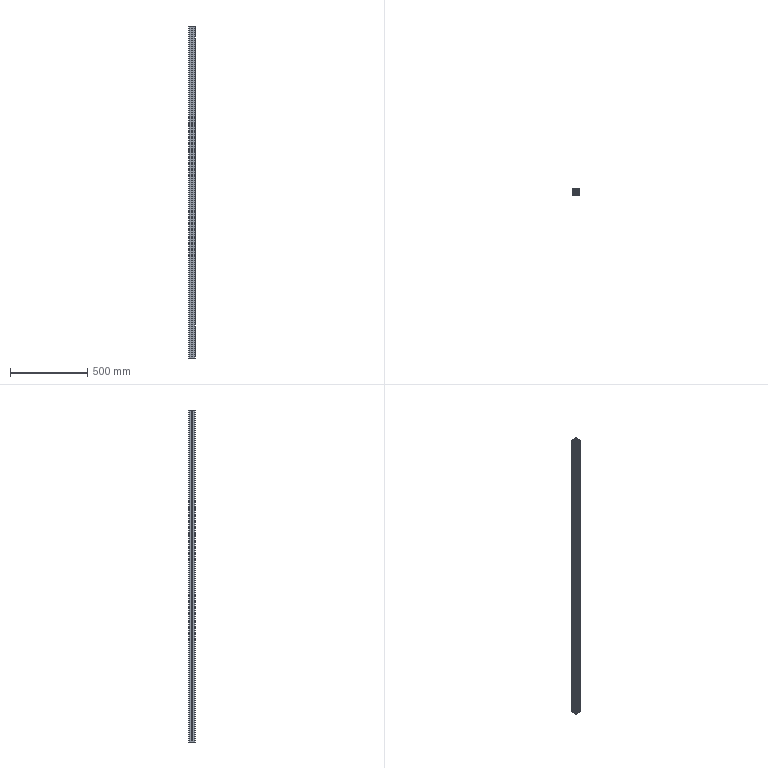Part | SolidWorks | features BaseBody 1, HoleWzd 1, MoveFace 1 | 1 solid | 320 faces | box 40 x 40 x 2150 mm | volume 1150023 mm3 | plane 214 | cylinder 106 | commonest cylinder face diameters 0.6 x24 9 x24 6.8 x20 10 x20 2 x8 15 x6